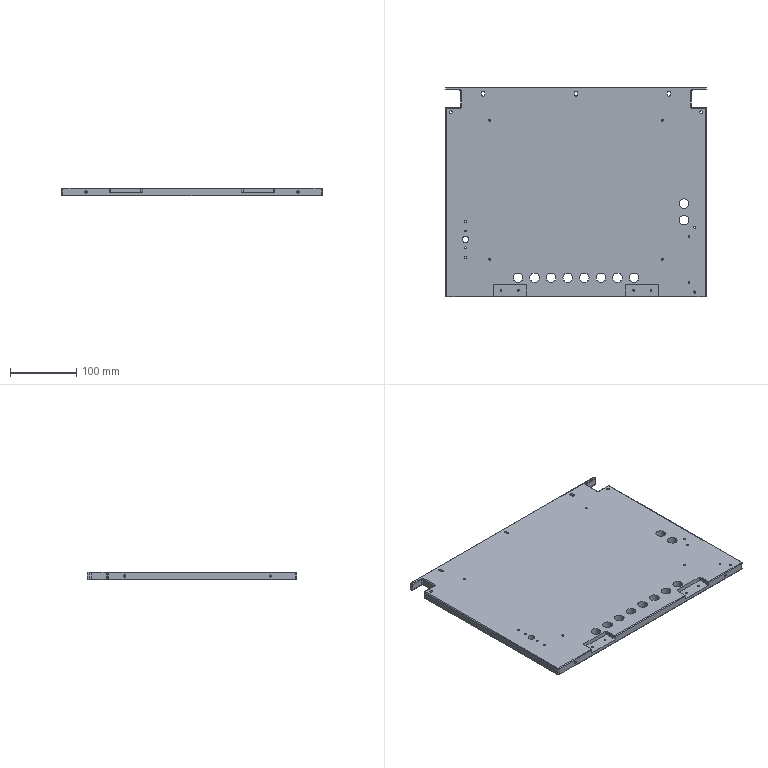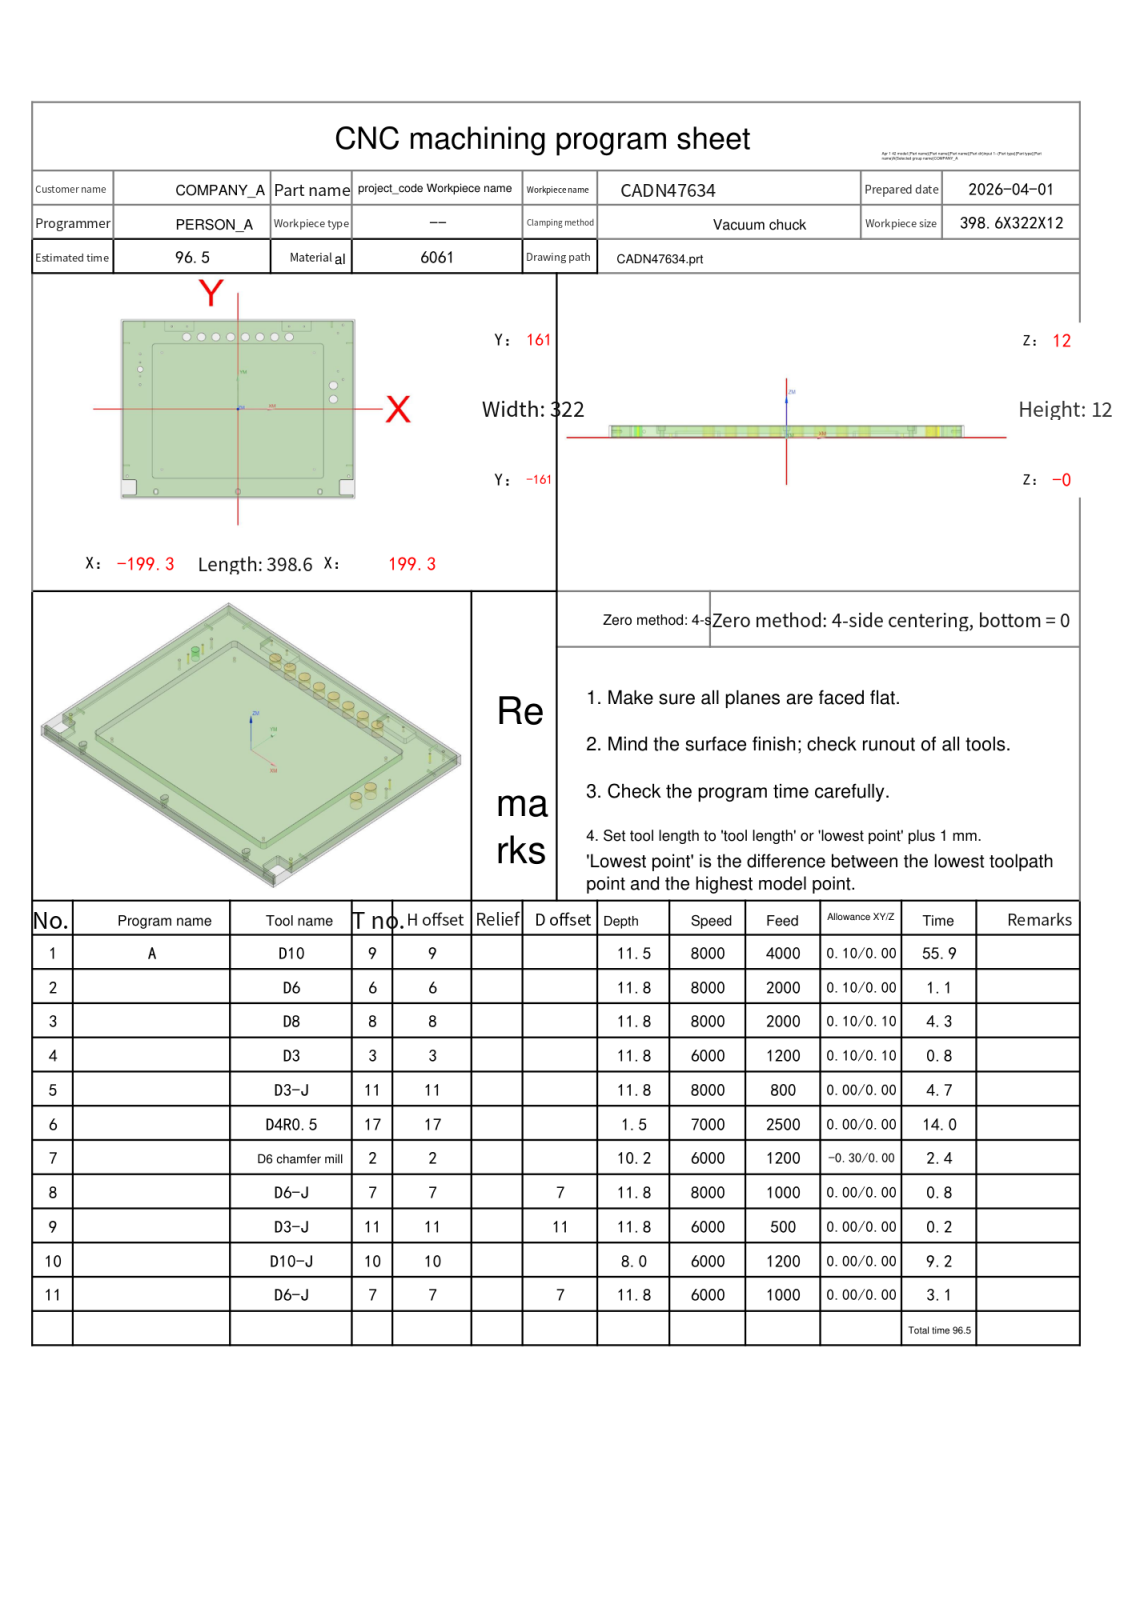NC program | NX | posted by the shop | part box 393.6 x 317 x 12 mm
Lines 4964 to 5551 of 16012:
N4 T03 M06
(D3  D=3. R=0. H=03 ce=0.10 di=0.10)
G00 G90 G54 X139.35 Y-148.5 M03 S6000
G43 H03 Z32.
M08
Z7.5
G01 Y-150. Z7.464 F1200.
G03 X140. Y-150.65 Z7.439 I.65 J0.0
X140.65 Y-150. Z7.415 I0.0 J.65
G01 Y-147. Z7.342
G03 X140. Y-146.35 Z7.318 I-.65 J0.0
X139.35 Y-147. Z7.293 I0.0 J-.65
G01 Y-150. Z7.22
G03 X140. Y-150.65 Z7.196 I.65 J0.0
X140.65 Y-150. Z7.171 I0.0 J.65
G01 Y-147. Z7.099
G03 X140. Y-146.35 Z7.074 I-.65 J0.0
X139.35 Y-147. Z7.05 I0.0 J-.65
G01 Y-150. Z6.977
G03 X140. Y-150.65 Z6.953 I.65 J0.0
X140.65 Y-150. Z6.928 I0.0 J.65
G01 Y-147. Z6.855
G03 X140. Y-146.35 Z6.831 I-.65 J0.0
X139.35 Y-147. Z6.806 I0.0 J-.65
G01 Y-150. Z6.734
G03 X140. Y-150.65 Z6.709 I.65 J0.0
X140.65 Y-150. Z6.685 I0.0 J.65
G01 Y-147. Z6.612
G03 X140. Y-146.35 Z6.588 I-.65 J0.0
X139.35 Y-147. Z6.563 I0.0 J-.65
G01 Y-150. Z6.49
G03 X140. Y-150.65 Z6.466 I.65 J0.0
X140.65 Y-150. Z6.441 I0.0 J.65
G01 Y-147. Z6.369
G03 X140. Y-146.35 Z6.344 I-.65 J0.0
X139.35 Y-147. Z6.32 I0.0 J-.65
G01 Y-150. Z6.247
G03 X140. Y-150.65 Z6.223 I.65 J0.0
X140.65 Y-150. Z6.198 I0.0 J.65
G01 Y-147. Z6.125
G03 X140. Y-146.35 Z6.101 I-.65 J0.0
X139.35 Y-147. Z6.076 I0.0 J-.65
G01 Y-150. Z6.004
G03 X140. Y-150.65 Z5.979 I.65 J0.0
X140.65 Y-150. Z5.955 I0.0 J.65
G01 Y-147. Z5.882
G03 X140. Y-146.35 Z5.858 I-.65 J0.0
X139.35 Y-147. Z5.833 I0.0 J-.65
G01 Y-150. Z5.76
G03 X140. Y-150.65 Z5.736 I.65 J0.0
X140.65 Y-150. Z5.711 I0.0 J.65
G01 Y-147. Z5.639
G03 X140. Y-146.35 Z5.614 I-.65 J0.0
X139.35 Y-147. Z5.59 I0.0 J-.65
G01 Y-150. Z5.517
G03 X140. Y-150.65 Z5.493 I.65 J0.0
X140.65 Y-150. Z5.468 I0.0 J.65
G01 Y-147. Z5.395
G03 X140. Y-146.35 Z5.371 I-.65 J0.0
X139.35 Y-147. Z5.346 I0.0 J-.65
G01 Y-150. Z5.274
G03 X140. Y-150.65 Z5.249 I.65 J0.0
X140.65 Y-150. Z5.225 I0.0 J.65
G01 Y-147. Z5.152
G03 X140. Y-146.35 Z5.128 I-.65 J0.0
X139.35 Y-147. Z5.103 I0.0 J-.65
G01 Y-150. Z5.03
G03 X140. Y-150.65 Z5.006 I.65 J0.0
X140.65 Y-150. Z4.981 I0.0 J.65
G01 Y-147. Z4.909
G03 X140. Y-146.35 Z4.884 I-.65 J0.0
X139.35 Y-147. Z4.86 I0.0 J-.65
G01 Y-150. Z4.787
G03 X140. Y-150.65 Z4.763 I.65 J0.0
X140.65 Y-150. Z4.738 I0.0 J.65
G01 Y-147. Z4.665
G03 X140. Y-146.35 Z4.641 I-.65 J0.0
X139.35 Y-147. Z4.616 I0.0 J-.65
G01 Y-150. Z4.544
G03 X140. Y-150.65 Z4.519 I.65 J0.0
X140.65 Y-150. Z4.495 I0.0 J.65
G01 Y-147. Z4.422
G03 X140. Y-146.35 Z4.398 I-.65 J0.0
X139.35 Y-147. Z4.373 I0.0 J-.65
G01 Y-150. Z4.3
G03 X140. Y-150.65 Z4.276 I.65 J0.0
X140.65 Y-150. Z4.251 I0.0 J.65
G01 Y-147. Z4.179
G03 X140. Y-146.35 Z4.154 I-.65 J0.0
X139.35 Y-147. Z4.13 I0.0 J-.65
G01 Y-150. Z4.057
G03 X140. Y-150.65 Z4.033 I.65 J0.0
X140.65 Y-150. Z4.008 I0.0 J.65
G01 Y-147. Z3.935
G03 X140. Y-146.35 Z3.911 I-.65 J0.0
X139.35 Y-147. Z3.886 I0.0 J-.65
G01 Y-150. Z3.814
G03 X140. Y-150.65 Z3.789 I.65 J0.0
X140.65 Y-150. Z3.765 I0.0 J.65
G01 Y-147. Z3.692
G03 X140. Y-146.35 Z3.668 I-.65 J0.0
X139.35 Y-147. Z3.643 I0.0 J-.65
G01 Y-150. Z3.57
G03 X140. Y-150.65 Z3.546 I.65 J0.0
X140.65 Y-150. Z3.521 I0.0 J.65
G01 Y-147. Z3.449
G03 X140. Y-146.35 Z3.424 I-.65 J0.0
X139.35 Y-147. Z3.4 I0.0 J-.65
G01 Y-150. Z3.327
G03 X140. Y-150.65 Z3.303 I.65 J0.0
X140.65 Y-150. Z3.278 I0.0 J.65
G01 Y-147. Z3.205
G03 X140. Y-146.35 Z3.181 I-.65 J0.0
X139.35 Y-147. Z3.156 I0.0 J-.65
G01 Y-150. Z3.084
G03 X140. Y-150.65 Z3.059 I.65 J0.0
X140.65 Y-150. Z3.035 I0.0 J.65
G01 Y-147. Z2.962
G03 X140. Y-146.35 Z2.938 I-.65 J0.0
X139.35 Y-147. Z2.913 I0.0 J-.65
G01 Y-150. Z2.84
G03 X140. Y-150.65 Z2.816 I.65 J0.0
X140.65 Y-150. Z2.791 I0.0 J.65
G01 Y-147. Z2.719
G03 X140. Y-146.35 Z2.694 I-.65 J0.0
X139.35 Y-147. Z2.67 I0.0 J-.65
G01 Y-150. Z2.597
G03 X140. Y-150.65 Z2.573 I.65 J0.0
X140.65 Y-150. Z2.548 I0.0 J.65
G01 Y-147. Z2.475
G03 X140. Y-146.35 Z2.451 I-.65 J0.0
X139.35 Y-147. Z2.426 I0.0 J-.65
G01 Y-150. Z2.354
G03 X140. Y-150.65 Z2.329 I.65 J0.0
X140.65 Y-150. Z2.305 I0.0 J.65
G01 Y-147. Z2.232
G03 X140. Y-146.35 Z2.208 I-.65 J0.0
X139.35 Y-147. Z2.183 I0.0 J-.65
G01 Y-150. Z2.11
G03 X140. Y-150.65 Z2.086 I.65 J0.0
X140.65 Y-150. Z2.061 I0.0 J.65
G01 Y-147. Z1.989
G03 X140. Y-146.35 Z1.964 I-.65 J0.0
X139.35 Y-147. Z1.94 I0.0 J-.65
G01 Y-150. Z1.867
G03 X140. Y-150.65 Z1.843 I.65 J0.0
X140.65 Y-150. Z1.818 I0.0 J.65
G01 Y-147. Z1.745
G03 X140. Y-146.35 Z1.721 I-.65 J0.0
X139.35 Y-147. Z1.696 I0.0 J-.65
G01 Y-150. Z1.624
G03 X140. Y-150.65 Z1.599 I.65 J0.0
X140.65 Y-150. Z1.575 I0.0 J.65
G01 Y-147. Z1.502
G03 X140. Y-146.35 Z1.478 I-.65 J0.0
X139.35 Y-147. Z1.453 I0.0 J-.65
G01 Y-150. Z1.38
G03 X140. Y-150.65 Z1.356 I.65 J0.0
X140.65 Y-150. Z1.331 I0.0 J.65
G01 Y-147. Z1.259
G03 X140. Y-146.35 Z1.234 I-.65 J0.0
X139.35 Y-147. Z1.21 I0.0 J-.65
G01 Y-150. Z1.137
G03 X140. Y-150.65 Z1.113 I.65 J0.0
X140.65 Y-150. Z1.088 I0.0 J.65
G01 Y-147. Z1.015
G03 X140. Y-146.35 Z.991 I-.65 J0.0
X139.35 Y-147. Z.966 I0.0 J-.65
G01 Y-150. Z.894
G03 X140. Y-150.65 Z.869 I.65 J0.0
X140.65 Y-150. Z.845 I0.0 J.65
G01 Y-147. Z.772
G03 X140. Y-146.35 Z.748 I-.65 J0.0
X139.35 Y-147. Z.723 I0.0 J-.65
G01 Y-150. Z.65
G03 X140. Y-150.65 Z.626 I.65 J0.0
X140.65 Y-150. Z.601 I0.0 J.65
G01 Y-147. Z.529
G03 X140. Y-146.35 Z.504 I-.65 J0.0
X139.35 Y-147. Z.48 I0.0 J-.65
G01 Y-150. Z.407
G03 X140. Y-150.65 Z.383 I.65 J0.0
X140.65 Y-150. Z.358 I0.0 J.65
G01 Y-147. Z.285
G03 X140. Y-146.35 Z.261 I-.65 J0.0
X139.35 Y-147. Z.236 I0.0 J-.65
G01 Y-148.5 Z.2
Y-150.
G03 X140. Y-150.65 I.65 J0.0
X140.65 Y-150. I0.0 J.65
G01 Y-147.
G03 X140. Y-146.35 I-.65 J0.0
X139.35 Y-147. I0.0 J-.65
G01 Y-148.5
Y-149.
Z1.2
G00 Z32.
X.65 Y-148.5
Z7.5
G01 Y-147. Z7.464
G03 X0.0 Y-146.35 Z7.439 I-.65 J0.0
X-.65 Y-147. Z7.415 I0.0 J-.65
G01 Y-150. Z7.342
G03 X0.0 Y-150.65 Z7.318 I.65 J0.0
X.65 Y-150. Z7.293 I0.0 J.65
G01 Y-147. Z7.22
G03 X0.0 Y-146.35 Z7.196 I-.65 J0.0
X-.65 Y-147. Z7.171 I0.0 J-.65
G01 Y-150. Z7.099
G03 X0.0 Y-150.65 Z7.074 I.65 J0.0
X.65 Y-150. Z7.05 I0.0 J.65
G01 Y-147. Z6.977
G03 X0.0 Y-146.35 Z6.953 I-.65 J0.0
X-.65 Y-147. Z6.928 I0.0 J-.65
G01 Y-150. Z6.855
G03 X0.0 Y-150.65 Z6.831 I.65 J0.0
X.65 Y-150. Z6.806 I0.0 J.65
G01 Y-147. Z6.734
G03 X0.0 Y-146.35 Z6.709 I-.65 J0.0
X-.65 Y-147. Z6.685 I0.0 J-.65
G01 Y-150. Z6.612
G03 X0.0 Y-150.65 Z6.588 I.65 J0.0
X.65 Y-150. Z6.563 I0.0 J.65
G01 Y-147. Z6.49
G03 X0.0 Y-146.35 Z6.466 I-.65 J0.0
X-.65 Y-147. Z6.441 I0.0 J-.65
G01 Y-150. Z6.369
G03 X0.0 Y-150.65 Z6.344 I.65 J0.0
X.65 Y-150. Z6.32 I0.0 J.65
G01 Y-147. Z6.247
G03 X0.0 Y-146.35 Z6.223 I-.65 J0.0
X-.65 Y-147. Z6.198 I0.0 J-.65
G01 Y-150. Z6.125
G03 X0.0 Y-150.65 Z6.101 I.65 J0.0
X.65 Y-150. Z6.076 I0.0 J.65
G01 Y-147. Z6.004
G03 X0.0 Y-146.35 Z5.979 I-.65 J0.0
X-.65 Y-147. Z5.955 I0.0 J-.65
G01 Y-150. Z5.882
G03 X0.0 Y-150.65 Z5.858 I.65 J0.0
X.65 Y-150. Z5.833 I0.0 J.65
G01 Y-147. Z5.76
G03 X0.0 Y-146.35 Z5.736 I-.65 J0.0
X-.65 Y-147. Z5.711 I0.0 J-.65
G01 Y-150. Z5.639
G03 X0.0 Y-150.65 Z5.614 I.65 J0.0
X.65 Y-150. Z5.59 I0.0 J.65
G01 Y-147. Z5.517
G03 X0.0 Y-146.35 Z5.493 I-.65 J0.0
X-.65 Y-147. Z5.468 I0.0 J-.65
G01 Y-150. Z5.395
G03 X0.0 Y-150.65 Z5.371 I.65 J0.0
X.65 Y-150. Z5.346 I0.0 J.65
G01 Y-147. Z5.274
G03 X0.0 Y-146.35 Z5.249 I-.65 J0.0
X-.65 Y-147. Z5.225 I0.0 J-.65
G01 Y-150. Z5.152
G03 X0.0 Y-150.65 Z5.128 I.65 J0.0
X.65 Y-150. Z5.103 I0.0 J.65
G01 Y-147. Z5.03
G03 X0.0 Y-146.35 Z5.006 I-.65 J0.0
X-.65 Y-147. Z4.981 I0.0 J-.65
G01 Y-150. Z4.909
G03 X0.0 Y-150.65 Z4.884 I.65 J0.0
X.65 Y-150. Z4.86 I0.0 J.65
G01 Y-147. Z4.787
G03 X0.0 Y-146.35 Z4.763 I-.65 J0.0
X-.65 Y-147. Z4.738 I0.0 J-.65
G01 Y-150. Z4.665
G03 X0.0 Y-150.65 Z4.641 I.65 J0.0
X.65 Y-150. Z4.616 I0.0 J.65
G01 Y-147. Z4.544
G03 X0.0 Y-146.35 Z4.519 I-.65 J0.0
X-.65 Y-147. Z4.495 I0.0 J-.65
G01 Y-150. Z4.422
G03 X0.0 Y-150.65 Z4.398 I.65 J0.0
X.65 Y-150. Z4.373 I0.0 J.65
G01 Y-147. Z4.3
G03 X0.0 Y-146.35 Z4.276 I-.65 J0.0
X-.65 Y-147. Z4.251 I0.0 J-.65
G01 Y-150. Z4.179
G03 X0.0 Y-150.65 Z4.154 I.65 J0.0
X.65 Y-150. Z4.13 I0.0 J.65
G01 Y-147. Z4.057
G03 X0.0 Y-146.35 Z4.033 I-.65 J0.0
X-.65 Y-147. Z4.008 I0.0 J-.65
G01 Y-150. Z3.935
G03 X0.0 Y-150.65 Z3.911 I.65 J0.0
X.65 Y-150. Z3.886 I0.0 J.65
G01 Y-147. Z3.814
G03 X0.0 Y-146.35 Z3.789 I-.65 J0.0
X-.65 Y-147. Z3.765 I0.0 J-.65
G01 Y-150. Z3.692
G03 X0.0 Y-150.65 Z3.668 I.65 J0.0
X.65 Y-150. Z3.643 I0.0 J.65
G01 Y-147. Z3.57
G03 X0.0 Y-146.35 Z3.546 I-.65 J0.0
X-.65 Y-147. Z3.521 I0.0 J-.65
G01 Y-150. Z3.449
G03 X0.0 Y-150.65 Z3.424 I.65 J0.0
X.65 Y-150. Z3.4 I0.0 J.65
G01 Y-147. Z3.327
G03 X0.0 Y-146.35 Z3.303 I-.65 J0.0
X-.65 Y-147. Z3.278 I0.0 J-.65
G01 Y-150. Z3.205
G03 X0.0 Y-150.65 Z3.181 I.65 J0.0
X.65 Y-150. Z3.156 I0.0 J.65
G01 Y-147. Z3.084
G03 X0.0 Y-146.35 Z3.059 I-.65 J0.0
X-.65 Y-147. Z3.035 I0.0 J-.65
G01 Y-150. Z2.962
G03 X0.0 Y-150.65 Z2.938 I.65 J0.0
X.65 Y-150. Z2.913 I0.0 J.65
G01 Y-147. Z2.84
G03 X0.0 Y-146.35 Z2.816 I-.65 J0.0
X-.65 Y-147. Z2.791 I0.0 J-.65
G01 Y-150. Z2.719
G03 X0.0 Y-150.65 Z2.694 I.65 J0.0
X.65 Y-150. Z2.67 I0.0 J.65
G01 Y-147. Z2.597
G03 X0.0 Y-146.35 Z2.573 I-.65 J0.0
X-.65 Y-147. Z2.548 I0.0 J-.65
G01 Y-150. Z2.475
G03 X0.0 Y-150.65 Z2.451 I.65 J0.0
X.65 Y-150. Z2.426 I0.0 J.65
G01 Y-147. Z2.354
G03 X0.0 Y-146.35 Z2.329 I-.65 J0.0
X-.65 Y-147. Z2.305 I0.0 J-.65
G01 Y-150. Z2.232
G03 X0.0 Y-150.65 Z2.208 I.65 J0.0
X.65 Y-150. Z2.183 I0.0 J.65
G01 Y-147. Z2.11
G03 X0.0 Y-146.35 Z2.086 I-.65 J0.0
X-.65 Y-147. Z2.061 I0.0 J-.65
G01 Y-150. Z1.989
G03 X0.0 Y-150.65 Z1.964 I.65 J0.0
X.65 Y-150. Z1.94 I0.0 J.65
G01 Y-147. Z1.867
G03 X0.0 Y-146.35 Z1.843 I-.65 J0.0
X-.65 Y-147. Z1.818 I0.0 J-.65
G01 Y-150. Z1.745
G03 X0.0 Y-150.65 Z1.721 I.65 J0.0
X.65 Y-150. Z1.696 I0.0 J.65
G01 Y-147. Z1.624
G03 X0.0 Y-146.35 Z1.599 I-.65 J0.0
X-.65 Y-147. Z1.575 I0.0 J-.65
G01 Y-150. Z1.502
G03 X0.0 Y-150.65 Z1.478 I.65 J0.0
X.65 Y-150. Z1.453 I0.0 J.65
G01 Y-147. Z1.38
G03 X0.0 Y-146.35 Z1.356 I-.65 J0.0
X-.65 Y-147. Z1.331 I0.0 J-.65
G01 Y-150. Z1.259
G03 X0.0 Y-150.65 Z1.234 I.65 J0.0
X.65 Y-150. Z1.21 I0.0 J.65
G01 Y-147. Z1.137
G03 X0.0 Y-146.35 Z1.113 I-.65 J0.0
X-.65 Y-147. Z1.088 I0.0 J-.65
G01 Y-150. Z1.015
G03 X0.0 Y-150.65 Z.991 I.65 J0.0
X.65 Y-150. Z.966 I0.0 J.65
G01 Y-147. Z.894
G03 X0.0 Y-146.35 Z.869 I-.65 J0.0
X-.65 Y-147. Z.845 I0.0 J-.65
G01 Y-150. Z.772
G03 X0.0 Y-150.65 Z.748 I.65 J0.0
X.65 Y-150. Z.723 I0.0 J.65
G01 Y-147. Z.65
G03 X0.0 Y-146.35 Z.626 I-.65 J0.0
X-.65 Y-147. Z.601 I0.0 J-.65
G01 Y-150. Z.529
G03 X0.0 Y-150.65 Z.504 I.65 J0.0
X.65 Y-150. Z.48 I0.0 J.65
G01 Y-147. Z.407
G03 X0.0 Y-146.35 Z.383 I-.65 J0.0
X-.65 Y-147. Z.358 I0.0 J-.65
G01 Y-150. Z.285
G03 X0.0 Y-150.65 Z.261 I.65 J0.0
X.65 Y-150. Z.236 I0.0 J.65
G01 Y-148.5 Z.2
Y-147.
G03 X0.0 Y-146.35 I-.65 J0.0
X-.65 Y-147. I0.0 J-.65
G01 Y-150.
G03 X0.0 Y-150.65 I.65 J0.0
X.65 Y-150. I0.0 J.65
G01 Y-148.5
Y-148.
Z1.2
G00 Z32.
X-139.35 Y-148.5
Z7.5
G01 Y-147. Z7.464
G03 X-140. Y-146.35 Z7.439 I-.65 J0.0
X-140.65 Y-147. Z7.415 I0.0 J-.65
G01 Y-150. Z7.342
G03 X-140. Y-150.65 Z7.318 I.65 J0.0
X-139.35 Y-150. Z7.293 I0.0 J.65
G01 Y-147. Z7.22
G03 X-140. Y-146.35 Z7.196 I-.65 J0.0
X-140.65 Y-147. Z7.171 I0.0 J-.65
G01 Y-150. Z7.099
G03 X-140. Y-150.65 Z7.074 I.65 J0.0
X-139.35 Y-150. Z7.05 I0.0 J.65
G01 Y-147. Z6.977
G03 X-140. Y-146.35 Z6.953 I-.65 J0.0
X-140.65 Y-147. Z6.928 I0.0 J-.65
G01 Y-150. Z6.855
G03 X-140. Y-150.65 Z6.831 I.65 J0.0
X-139.35 Y-150. Z6.806 I0.0 J.65
G01 Y-147. Z6.734
G03 X-140. Y-146.35 Z6.709 I-.65 J0.0
X-140.65 Y-147. Z6.685 I0.0 J-.65
G01 Y-150. Z6.612
G03 X-140. Y-150.65 Z6.588 I.65 J0.0
X-139.35 Y-150. Z6.563 I0.0 J.65
G01 Y-147. Z6.49
G03 X-140. Y-146.35 Z6.466 I-.65 J0.0
X-140.65 Y-147. Z6.441 I0.0 J-.65
G01 Y-150. Z6.369
G03 X-140. Y-150.65 Z6.344 I.65 J0.0
X-139.35 Y-150. Z6.32 I0.0 J.65
G01 Y-147. Z6.247
G03 X-140. Y-146.35 Z6.223 I-.65 J0.0
X-140.65 Y-147. Z6.198 I0.0 J-.65
G01 Y-150. Z6.125
G03 X-140. Y-150.65 Z6.101 I.65 J0.0
X-139.35 Y-150. Z6.076 I0.0 J.65
G01 Y-147. Z6.004
G03 X-140. Y-146.35 Z5.979 I-.65 J0.0
X-140.65 Y-147. Z5.955 I0.0 J-.65
G01 Y-150. Z5.882
G03 X-140. Y-150.65 Z5.858 I.65 J0.0
X-139.35 Y-150. Z5.833 I0.0 J.65
G01 Y-147. Z5.76
G03 X-140. Y-146.35 Z5.736 I-.65 J0.0
X-140.65 Y-147. Z5.711 I0.0 J-.65
G01 Y-150. Z5.639
G03 X-140. Y-150.65 Z5.614 I.65 J0.0
X-139.35 Y-150. Z5.59 I0.0 J.65
G01 Y-147. Z5.517
G03 X-140. Y-146.35 Z5.493 I-.65 J0.0
X-140.65 Y-147. Z5.468 I0.0 J-.65
G01 Y-150. Z5.395
G03 X-140. Y-150.65 Z5.371 I.65 J0.0
X-139.35 Y-150. Z5.346 I0.0 J.65
G01 Y-147. Z5.274
G03 X-140. Y-146.35 Z5.249 I-.65 J0.0
X-140.65 Y-147. Z5.225 I0.0 J-.65
G01 Y-150. Z5.152
G03 X-140. Y-150.65 Z5.128 I.65 J0.0
X-139.35 Y-150. Z5.103 I0.0 J.65
G01 Y-147. Z5.03
G03 X-140. Y-146.35 Z5.006 I-.65 J0.0
X-140.65 Y-147. Z4.981 I0.0 J-.65
G01 Y-150. Z4.909
G03 X-140. Y-150.65 Z4.884 I.65 J0.0
X-139.35 Y-150. Z4.86 I0.0 J.65
G01 Y-147. Z4.787
G03 X-140. Y-146.35 Z4.763 I-.65 J0.0
X-140.65 Y-147. Z4.738 I0.0 J-.65
G01 Y-150. Z4.665
G03 X-140. Y-150.65 Z4.641 I.65 J0.0
X-139.35 Y-150. Z4.616 I0.0 J.65
G01 Y-147. Z4.544
G03 X-140. Y-146.35 Z4.519 I-.65 J0.0
X-140.65 Y-147. Z4.495 I0.0 J-.65
G01 Y-150. Z4.422
G03 X-140. Y-150.65 Z4.398 I.65 J0.0
X-139.35 Y-150. Z4.373 I0.0 J.65
G01 Y-147. Z4.3
G03 X-140. Y-146.35 Z4.276 I-.65 J0.0
X-140.65 Y-147. Z4.251 I0.0 J-.65
G01 Y-150. Z4.179
G03 X-140. Y-150.65 Z4.154 I.65 J0.0
X-139.35 Y-150. Z4.13 I0.0 J.65
G01 Y-147. Z4.057
G03 X-140. Y-146.35 Z4.033 I-.65 J0.0
X-140.65 Y-147. Z4.008 I0.0 J-.65
G01 Y-150. Z3.935
G03 X-140. Y-150.65 Z3.911 I.65 J0.0
X-139.35 Y-150. Z3.886 I0.0 J.65
G01 Y-147. Z3.814
G03 X-140. Y-146.35 Z3.789 I-.65 J0.0
X-140.65 Y-147. Z3.765 I0.0 J-.65
G01 Y-150. Z3.692
G03 X-140. Y-150.65 Z3.668 I.65 J0.0
X-139.35 Y-150. Z3.643 I0.0 J.65
G01 Y-147. Z3.57
G03 X-140. Y-146.35 Z3.546 I-.65 J0.0
X-140.65 Y-147. Z3.521 I0.0 J-.65
G01 Y-150. Z3.449
G03 X-140. Y-150.65 Z3.424 I.65 J0.0
X-139.35 Y-150. Z3.4 I0.0 J.65
G01 Y-147. Z3.327
G03 X-140. Y-146.35 Z3.303 I-.65 J0.0
X-140.65 Y-147. Z3.278 I0.0 J-.65
G01 Y-150. Z3.205
G03 X-140. Y-150.65 Z3.181 I.65 J0.0
X-139.35 Y-150. Z3.156 I0.0 J.65
G01 Y-147. Z3.084
G03 X-140. Y-146.35 Z3.059 I-.65 J0.0
X-140.65 Y-147. Z3.035 I0.0 J-.65
G01 Y-150. Z2.962
G03 X-140. Y-150.65 Z2.938 I.65 J0.0
X-139.35 Y-150. Z2.913 I0.0 J.65
G01 Y-147. Z2.84
G03 X-140. Y-146.35 Z2.816 I-.65 J0.0
X-140.65 Y-147. Z2.791 I0.0 J-.65
G01 Y-150. Z2.719
G03 X-140. Y-150.65 Z2.694 I.65 J0.0
X-139.35 Y-150. Z2.67 I0.0 J.65
G01 Y-147. Z2.597
G03 X-140. Y-146.35 Z2.573 I-.65 J0.0
X-140.65 Y-147. Z2.548 I0.0 J-.65
G01 Y-150. Z2.475
G03 X-140. Y-150.65 Z2.451 I.65 J0.0
X-139.35 Y-150. Z2.426 I0.0 J.65
G01 Y-147. Z2.354
G03 X-140. Y-146.35 Z2.329 I-.65 J0.0
X-140.65 Y-147. Z2.305 I0.0 J-.65
G01 Y-150. Z2.232
G03 X-140. Y-150.65 Z2.208 I.65 J0.0
X-139.35 Y-150. Z2.183 I0.0 J.65
G01 Y-147. Z2.11
G03 X-140. Y-146.35 Z2.086 I-.65 J0.0
X-140.65 Y-147. Z2.061 I0.0 J-.65
G01 Y-150. Z1.989
G03 X-140. Y-150.65 Z1.964 I.65 J0.0
X-139.35 Y-150. Z1.94 I0.0 J.65
G01 Y-147. Z1.867
G03 X-140. Y-146.35 Z1.843 I-.65 J0.0
X-140.65 Y-147. Z1.818 I0.0 J-.65
G01 Y-150. Z1.745
G03 X-140. Y-150.65 Z1.721 I.65 J0.0
X-139.35 Y-150. Z1.696 I0.0 J.65
G01 Y-147. Z1.624
G03 X-140. Y-146.35 Z1.599 I-.65 J0.0
X-140.65 Y-147. Z1.575 I0.0 J-.65
G01 Y-150. Z1.502
G03 X-140. Y-150.65 Z1.478 I.65 J0.0
X-139.35 Y-150. Z1.453 I0.0 J.65
G01 Y-147. Z1.38
G03 X-140. Y-146.35 Z1.356 I-.65 J0.0
X-140.65 Y-147. Z1.331 I0.0 J-.65
G01 Y-150. Z1.259
G03 X-140. Y-150.65 Z1.234 I.65 J0.0
X-139.35 Y-150. Z1.21 I0.0 J.65
G01 Y-147. Z1.137
G03 X-140. Y-146.35 Z1.113 I-.65 J0.0
X-140.65 Y-147. Z1.088 I0.0 J-.65
G01 Y-150. Z1.015
G03 X-140. Y-150.65 Z.991 I.65 J0.0
X-139.35 Y-150. Z.966 I0.0 J.65
G01 Y-147. Z.894
G03 X-140. Y-146.35 Z.869 I-.65 J0.0
X-140.65 Y-147. Z.845 I0.0 J-.65
G01 Y-150. Z.772
G03 X-140. Y-150.65 Z.748 I.65 J0.0
X-139.35 Y-150. Z.723 I0.0 J.65
G01 Y-147. Z.65
G03 X-140. Y-146.35 Z.626 I-.65 J0.0
X-140.65 Y-147. Z.601 I0.0 J-.65
G01 Y-150. Z.529
G03 X-140. Y-150.65 Z.504 I.65 J0.0
X-139.35 Y-150. Z.48 I0.0 J.65
G01 Y-147. Z.407
G03 X-140. Y-146.35 Z.383 I-.65 J0.0
X-140.65 Y-147. Z.358 I0.0 J-.65
G01 Y-150. Z.285
G03 X-140. Y-150.65 Z.261 I.65 J0.0
X-139.35 Y-150. Z.236 I0.0 J.65
G01 Y-148.5 Z.2
Y-147.
G03 X-140. Y-146.35 I-.65 J0.0
X-140.65 Y-147. I0.0 J-.65
G01 Y-150.
G03 X-140. Y-150.65 I.65 J0.0
X-139.35 Y-150. I0.0 J.65
G01 Y-148.5
Y-148.
Z1.2
G00 Z32.
G91 G28 Z0.0
M05
M09
G91 G28 Z0.0
M01